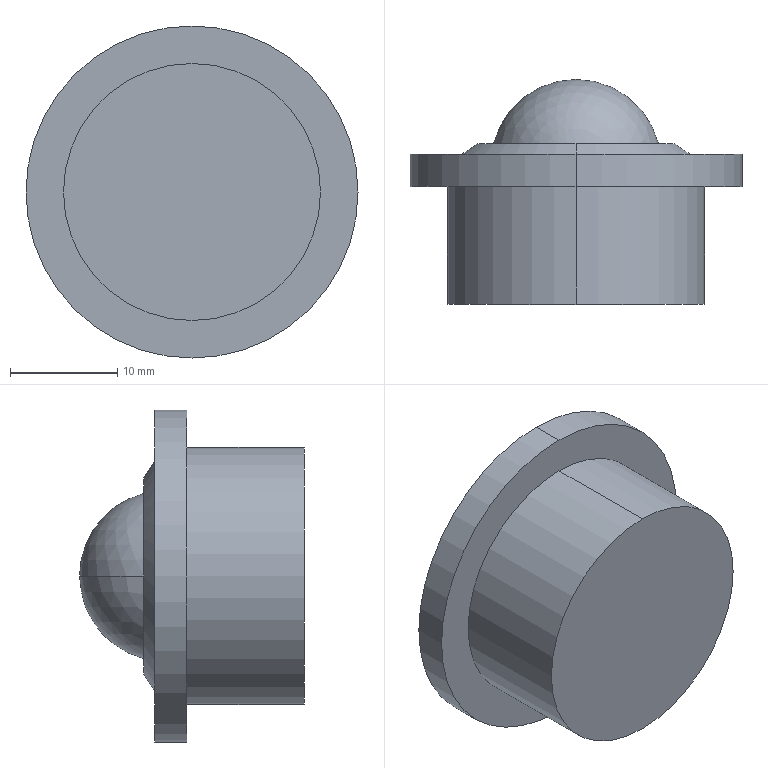Part | STEP file | Universal ball bearing H21xD31xh6-40KG | 1 solid | 12 faces | box 31 x 21 x 31 mm | volume 8224 mm3 | cylinder 4 | plane 4 | cone 2 | sphere 2 | commonest cylinder face diameters 24 x2 31 x2
STEP:
#1=CARTESIAN_POINT('',(0.,0.,0.));
#2=DIRECTION('',(0.,0.,1.));
#3=DIRECTION('',(1.,0.,0.));
#4=AXIS2_PLACEMENT_3D('',#1,#2,#3);
#5=CARTESIAN_POINT('',(0.,15.,-9.197));
#6=VERTEX_POINT('',#5);
#7=CARTESIAN_POINT('',(0.,15.,9.197));
#8=VERTEX_POINT('',#7);
#9=CARTESIAN_POINT('',(0.,15.,0.));
#10=DIRECTION('',(0.,-1.,0.));
#11=DIRECTION('',(0.,0.,-1.));
#12=AXIS2_PLACEMENT_3D('',#9,#10,#11);
#13=CIRCLE('',#12,9.197);
#14=CARTESIAN_POINT('',(0.,15.,0.));
#15=DIRECTION('',(0.,-1.,0.));
#16=DIRECTION('',(0.,0.,-1.));
#17=AXIS2_PLACEMENT_3D('',#14,#15,#16);
#18=CONICAL_SURFACE('',#17,9.197,0.9828);
#19=CARTESIAN_POINT('',(0.,0.));
#20=DIRECTION('',(1.,0.));
#21=VECTOR('',#20,1.);
#22=LINE('',#19,#21);
#23=(GEOMETRIC_REPRESENTATION_CONTEXT(2)PARAMETRIC_REPRESENTATION_CONTEXT()REPRESENTATION_CONTEXT('',''));
#24=DEFINITIONAL_REPRESENTATION('',(#22),#23);
#25=PCURVE('',#18,#24);
#26=CARTESIAN_POINT('',(0.,15.,0.));
#27=DIRECTION('',(0.,-1.,0.));
#28=DIRECTION('',(0.,0.,-1.));
#29=AXIS2_PLACEMENT_3D('',#26,#27,#28);
#30=PLANE('',#29);
#31=CARTESIAN_POINT('',(0.,0.));
#32=DIRECTION('',(1.,0.));
#33=AXIS2_PLACEMENT_2D('',#31,#32);
#34=CIRCLE('',#33,9.197);
#35=(GEOMETRIC_REPRESENTATION_CONTEXT(2)PARAMETRIC_REPRESENTATION_CONTEXT()REPRESENTATION_CONTEXT('',''));
#36=DEFINITIONAL_REPRESENTATION('',(#34),#35);
#37=PCURVE('',#30,#36);
#38=SURFACE_CURVE('',#13,(#25,#37),.PCURVE_S1.);
#39=EDGE_CURVE('',#6,#8,#38,.T.);
#40=ORIENTED_EDGE('',*,*,#39,.T.);
#41=CARTESIAN_POINT('',(0.,14.,10.697));
#42=VERTEX_POINT('',#41);
#43=CARTESIAN_POINT('',(0.,15.,9.197));
#44=DIRECTION('',(0.,-0.5547,0.8321));
#45=VECTOR('',#44,1.);
#46=LINE('',#43,#45);
#47=CARTESIAN_POINT('',(3.142,0.));
#48=DIRECTION('',(0.,1.));
#49=VECTOR('',#48,1.);
#50=LINE('',#47,#49);
#51=(GEOMETRIC_REPRESENTATION_CONTEXT(2)PARAMETRIC_REPRESENTATION_CONTEXT()REPRESENTATION_CONTEXT('',''));
#52=DEFINITIONAL_REPRESENTATION('',(#50),#51);
#53=PCURVE('',#18,#52);
#54=CARTESIAN_POINT('',(0.,15.,0.));
#55=DIRECTION('',(0.,-1.,0.));
#56=DIRECTION('',(0.,0.,-1.));
#57=AXIS2_PLACEMENT_3D('',#54,#55,#56);
#58=CONICAL_SURFACE('',#57,9.197,0.9828);
#59=CARTESIAN_POINT('',(3.142,0.));
#60=DIRECTION('',(0.,1.));
#61=VECTOR('',#60,1.);
#62=LINE('',#59,#61);
#63=(GEOMETRIC_REPRESENTATION_CONTEXT(2)PARAMETRIC_REPRESENTATION_CONTEXT()REPRESENTATION_CONTEXT('',''));
#64=DEFINITIONAL_REPRESENTATION('',(#62),#63);
#65=PCURVE('',#58,#64);
#66=SURFACE_CURVE('',#46,(#53,#65),.PCURVE_S1.);
#67=EDGE_CURVE('',#8,#42,#66,.T.);
#68=ORIENTED_EDGE('',*,*,#67,.T.);
#69=CARTESIAN_POINT('',(0.,14.,-10.697));
#70=VERTEX_POINT('',#69);
#71=CARTESIAN_POINT('',(0.,14.,0.));
#72=DIRECTION('',(0.,-1.,0.));
#73=DIRECTION('',(0.,0.,-1.));
#74=AXIS2_PLACEMENT_3D('',#71,#72,#73);
#75=CIRCLE('',#74,10.697);
#76=CARTESIAN_POINT('',(0.,1.));
#77=DIRECTION('',(1.,0.));
#78=VECTOR('',#77,1.);
#79=LINE('',#76,#78);
#80=(GEOMETRIC_REPRESENTATION_CONTEXT(2)PARAMETRIC_REPRESENTATION_CONTEXT()REPRESENTATION_CONTEXT('',''));
#81=DEFINITIONAL_REPRESENTATION('',(#79),#80);
#82=PCURVE('',#18,#81);
#83=CARTESIAN_POINT('',(0.,14.,0.));
#84=DIRECTION('',(0.,-1.,0.));
#85=DIRECTION('',(0.,0.,-1.));
#86=AXIS2_PLACEMENT_3D('',#83,#84,#85);
#87=PLANE('',#86);
#88=CARTESIAN_POINT('',(0.,0.));
#89=DIRECTION('',(1.,0.));
#90=AXIS2_PLACEMENT_2D('',#88,#89);
#91=CIRCLE('',#90,10.697);
#92=(GEOMETRIC_REPRESENTATION_CONTEXT(2)PARAMETRIC_REPRESENTATION_CONTEXT()REPRESENTATION_CONTEXT('',''));
#93=DEFINITIONAL_REPRESENTATION('',(#91),#92);
#94=PCURVE('',#87,#93);
#95=SURFACE_CURVE('',#75,(#82,#94),.PCURVE_S1.);
#96=EDGE_CURVE('',#70,#42,#95,.T.);
#97=ORIENTED_EDGE('',*,*,#96,.F.);
#98=CARTESIAN_POINT('',(0.,15.,-9.197));
#99=DIRECTION('',(0.,-0.5547,-0.8321));
#100=VECTOR('',#99,1.);
#101=LINE('',#98,#100);
#102=CARTESIAN_POINT('',(0.,0.));
#103=DIRECTION('',(0.,1.));
#104=VECTOR('',#103,1.);
#105=LINE('',#102,#104);
#106=(GEOMETRIC_REPRESENTATION_CONTEXT(2)PARAMETRIC_REPRESENTATION_CONTEXT()REPRESENTATION_CONTEXT('',''));
#107=DEFINITIONAL_REPRESENTATION('',(#105),#106);
#108=PCURVE('',#18,#107);
#109=CARTESIAN_POINT('',(6.283,0.));
#110=DIRECTION('',(0.,1.));
#111=VECTOR('',#110,1.);
#112=LINE('',#109,#111);
#113=(GEOMETRIC_REPRESENTATION_CONTEXT(2)PARAMETRIC_REPRESENTATION_CONTEXT()REPRESENTATION_CONTEXT('',''));
#114=DEFINITIONAL_REPRESENTATION('',(#112),#113);
#115=PCURVE('',#58,#114);
#116=SURFACE_CURVE('',#101,(#108,#115),.PCURVE_S1.);
#117=EDGE_CURVE('',#6,#70,#116,.T.);
#118=ORIENTED_EDGE('',*,*,#117,.F.);
#119=EDGE_LOOP('',(#40,#68,#97,#118));
#120=FACE_BOUND('',#119,.T.);
#121=ADVANCED_FACE('',(#120),#18,.T.);
#122=CARTESIAN_POINT('',(0.,14.,-15.5));
#123=VERTEX_POINT('',#122);
#124=CARTESIAN_POINT('',(0.,14.,15.5));
#125=VERTEX_POINT('',#124);
#126=CARTESIAN_POINT('',(0.,14.,0.));
#127=DIRECTION('',(0.,-1.,0.));
#128=DIRECTION('',(0.,0.,-1.));
#129=AXIS2_PLACEMENT_3D('',#126,#127,#128);
#130=CIRCLE('',#129,15.5);
#131=CARTESIAN_POINT('',(0.,0.,0.));
#132=DIRECTION('',(0.,-1.,0.));
#133=DIRECTION('',(0.,0.,-1.));
#134=AXIS2_PLACEMENT_3D('',#131,#132,#133);
#135=CYLINDRICAL_SURFACE('',#134,15.5);
#136=CARTESIAN_POINT('',(0.,-14.));
#137=DIRECTION('',(1.,0.));
#138=VECTOR('',#137,1.);
#139=LINE('',#136,#138);
#140=(GEOMETRIC_REPRESENTATION_CONTEXT(2)PARAMETRIC_REPRESENTATION_CONTEXT()REPRESENTATION_CONTEXT('',''));
#141=DEFINITIONAL_REPRESENTATION('',(#139),#140);
#142=PCURVE('',#135,#141);
#143=CARTESIAN_POINT('',(0.,0.));
#144=DIRECTION('',(1.,0.));
#145=AXIS2_PLACEMENT_2D('',#143,#144);
#146=CIRCLE('',#145,15.5);
#147=(GEOMETRIC_REPRESENTATION_CONTEXT(2)PARAMETRIC_REPRESENTATION_CONTEXT()REPRESENTATION_CONTEXT('',''));
#148=DEFINITIONAL_REPRESENTATION('',(#146),#147);
#149=PCURVE('',#87,#148);
#150=SURFACE_CURVE('',#130,(#142,#149),.PCURVE_S1.);
#151=EDGE_CURVE('',#123,#125,#150,.T.);
#152=ORIENTED_EDGE('',*,*,#151,.T.);
#153=CARTESIAN_POINT('',(0.,11.,15.5));
#154=VERTEX_POINT('',#153);
#155=CARTESIAN_POINT('',(0.,0.,15.5));
#156=DIRECTION('',(0.,-1.,0.));
#157=VECTOR('',#156,1.);
#158=LINE('',#155,#157);
#159=CARTESIAN_POINT('',(3.142,0.));
#160=DIRECTION('',(0.,1.));
#161=VECTOR('',#160,1.);
#162=LINE('',#159,#161);
#163=(GEOMETRIC_REPRESENTATION_CONTEXT(2)PARAMETRIC_REPRESENTATION_CONTEXT()REPRESENTATION_CONTEXT('',''));
#164=DEFINITIONAL_REPRESENTATION('',(#162),#163);
#165=PCURVE('',#135,#164);
#166=CARTESIAN_POINT('',(0.,0.,0.));
#167=DIRECTION('',(0.,-1.,0.));
#168=DIRECTION('',(0.,0.,-1.));
#169=AXIS2_PLACEMENT_3D('',#166,#167,#168);
#170=CYLINDRICAL_SURFACE('',#169,15.5);
#171=CARTESIAN_POINT('',(3.142,0.));
#172=DIRECTION('',(0.,1.));
#173=VECTOR('',#172,1.);
#174=LINE('',#171,#173);
#175=(GEOMETRIC_REPRESENTATION_CONTEXT(2)PARAMETRIC_REPRESENTATION_CONTEXT()REPRESENTATION_CONTEXT('',''));
#176=DEFINITIONAL_REPRESENTATION('',(#174),#175);
#177=PCURVE('',#170,#176);
#178=SURFACE_CURVE('',#158,(#165,#177),.PCURVE_S1.);
#179=EDGE_CURVE('',#125,#154,#178,.T.);
#180=ORIENTED_EDGE('',*,*,#179,.T.);
#181=CARTESIAN_POINT('',(0.,11.,-15.5));
#182=VERTEX_POINT('',#181);
#183=CARTESIAN_POINT('',(0.,11.,0.));
#184=DIRECTION('',(0.,-1.,0.));
#185=DIRECTION('',(0.,0.,-1.));
#186=AXIS2_PLACEMENT_3D('',#183,#184,#185);
#187=CIRCLE('',#186,15.5);
#188=CARTESIAN_POINT('',(0.,-11.));
#189=DIRECTION('',(1.,0.));
#190=VECTOR('',#189,1.);
#191=LINE('',#188,#190);
#192=(GEOMETRIC_REPRESENTATION_CONTEXT(2)PARAMETRIC_REPRESENTATION_CONTEXT()REPRESENTATION_CONTEXT('',''));
#193=DEFINITIONAL_REPRESENTATION('',(#191),#192);
#194=PCURVE('',#135,#193);
#195=CARTESIAN_POINT('',(0.,11.,0.));
#196=DIRECTION('',(0.,-1.,0.));
#197=DIRECTION('',(0.,0.,-1.));
#198=AXIS2_PLACEMENT_3D('',#195,#196,#197);
#199=PLANE('',#198);
#200=CARTESIAN_POINT('',(0.,0.));
#201=DIRECTION('',(1.,0.));
#202=AXIS2_PLACEMENT_2D('',#200,#201);
#203=CIRCLE('',#202,15.5);
#204=(GEOMETRIC_REPRESENTATION_CONTEXT(2)PARAMETRIC_REPRESENTATION_CONTEXT()REPRESENTATION_CONTEXT('',''));
#205=DEFINITIONAL_REPRESENTATION('',(#203),#204);
#206=PCURVE('',#199,#205);
#207=SURFACE_CURVE('',#187,(#194,#206),.PCURVE_S1.);
#208=EDGE_CURVE('',#182,#154,#207,.T.);
#209=ORIENTED_EDGE('',*,*,#208,.F.);
#210=CARTESIAN_POINT('',(0.,0.,-15.5));
#211=DIRECTION('',(0.,-1.,0.));
#212=VECTOR('',#211,1.);
#213=LINE('',#210,#212);
#214=CARTESIAN_POINT('',(0.,0.));
#215=DIRECTION('',(0.,1.));
#216=VECTOR('',#215,1.);
#217=LINE('',#214,#216);
#218=(GEOMETRIC_REPRESENTATION_CONTEXT(2)PARAMETRIC_REPRESENTATION_CONTEXT()REPRESENTATION_CONTEXT('',''));
#219=DEFINITIONAL_REPRESENTATION('',(#217),#218);
#220=PCURVE('',#135,#219);
#221=CARTESIAN_POINT('',(6.283,0.));
#222=DIRECTION('',(0.,1.));
#223=VECTOR('',#222,1.);
#224=LINE('',#221,#223);
#225=(GEOMETRIC_REPRESENTATION_CONTEXT(2)PARAMETRIC_REPRESENTATION_CONTEXT()REPRESENTATION_CONTEXT('',''));
#226=DEFINITIONAL_REPRESENTATION('',(#224),#225);
#227=PCURVE('',#170,#226);
#228=SURFACE_CURVE('',#213,(#220,#227),.PCURVE_S1.);
#229=EDGE_CURVE('',#123,#182,#228,.T.);
#230=ORIENTED_EDGE('',*,*,#229,.F.);
#231=EDGE_LOOP('',(#152,#180,#209,#230));
#232=FACE_BOUND('',#231,.T.);
#233=ADVANCED_FACE('',(#232),#135,.T.);
#234=CARTESIAN_POINT('',(0.,11.,-12.));
#235=VERTEX_POINT('',#234);
#236=CARTESIAN_POINT('',(0.,11.,12.));
#237=VERTEX_POINT('',#236);
#238=CARTESIAN_POINT('',(0.,11.,0.));
#239=DIRECTION('',(0.,-1.,0.));
#240=DIRECTION('',(0.,0.,-1.));
#241=AXIS2_PLACEMENT_3D('',#238,#239,#240);
#242=CIRCLE('',#241,12.);
#243=CARTESIAN_POINT('',(0.,0.,0.));
#244=DIRECTION('',(0.,-1.,0.));
#245=DIRECTION('',(0.,0.,-1.));
#246=AXIS2_PLACEMENT_3D('',#243,#244,#245);
#247=CYLINDRICAL_SURFACE('',#246,12.);
#248=CARTESIAN_POINT('',(0.,-11.));
#249=DIRECTION('',(1.,0.));
#250=VECTOR('',#249,1.);
#251=LINE('',#248,#250);
#252=(GEOMETRIC_REPRESENTATION_CONTEXT(2)PARAMETRIC_REPRESENTATION_CONTEXT()REPRESENTATION_CONTEXT('',''));
#253=DEFINITIONAL_REPRESENTATION('',(#251),#252);
#254=PCURVE('',#247,#253);
#255=CARTESIAN_POINT('',(0.,0.));
#256=DIRECTION('',(1.,0.));
#257=AXIS2_PLACEMENT_2D('',#255,#256);
#258=CIRCLE('',#257,12.);
#259=(GEOMETRIC_REPRESENTATION_CONTEXT(2)PARAMETRIC_REPRESENTATION_CONTEXT()REPRESENTATION_CONTEXT('',''));
#260=DEFINITIONAL_REPRESENTATION('',(#258),#259);
#261=PCURVE('',#199,#260);
#262=SURFACE_CURVE('',#242,(#254,#261),.PCURVE_S1.);
#263=EDGE_CURVE('',#235,#237,#262,.T.);
#264=ORIENTED_EDGE('',*,*,#263,.T.);
#265=CARTESIAN_POINT('',(0.,0.,12.));
#266=VERTEX_POINT('',#265);
#267=CARTESIAN_POINT('',(0.,0.,12.));
#268=DIRECTION('',(0.,-1.,0.));
#269=VECTOR('',#268,1.);
#270=LINE('',#267,#269);
#271=CARTESIAN_POINT('',(3.142,0.));
#272=DIRECTION('',(0.,1.));
#273=VECTOR('',#272,1.);
#274=LINE('',#271,#273);
#275=(GEOMETRIC_REPRESENTATION_CONTEXT(2)PARAMETRIC_REPRESENTATION_CONTEXT()REPRESENTATION_CONTEXT('',''));
#276=DEFINITIONAL_REPRESENTATION('',(#274),#275);
#277=PCURVE('',#247,#276);
#278=CARTESIAN_POINT('',(0.,0.,0.));
#279=DIRECTION('',(0.,-1.,0.));
#280=DIRECTION('',(0.,0.,-1.));
#281=AXIS2_PLACEMENT_3D('',#278,#279,#280);
#282=CYLINDRICAL_SURFACE('',#281,12.);
#283=CARTESIAN_POINT('',(3.142,0.));
#284=DIRECTION('',(0.,1.));
#285=VECTOR('',#284,1.);
#286=LINE('',#283,#285);
#287=(GEOMETRIC_REPRESENTATION_CONTEXT(2)PARAMETRIC_REPRESENTATION_CONTEXT()REPRESENTATION_CONTEXT('',''));
#288=DEFINITIONAL_REPRESENTATION('',(#286),#287);
#289=PCURVE('',#282,#288);
#290=SURFACE_CURVE('',#270,(#277,#289),.PCURVE_S1.);
#291=EDGE_CURVE('',#237,#266,#290,.T.);
#292=ORIENTED_EDGE('',*,*,#291,.T.);
#293=CARTESIAN_POINT('',(0.,0.,-12.));
#294=VERTEX_POINT('',#293);
#295=CARTESIAN_POINT('',(0.,0.,0.));
#296=DIRECTION('',(0.,-1.,0.));
#297=DIRECTION('',(0.,0.,-1.));
#298=AXIS2_PLACEMENT_3D('',#295,#296,#297);
#299=CIRCLE('',#298,12.);
#300=CARTESIAN_POINT('',(0.,0.));
#301=DIRECTION('',(1.,0.));
#302=VECTOR('',#301,1.);
#303=LINE('',#300,#302);
#304=(GEOMETRIC_REPRESENTATION_CONTEXT(2)PARAMETRIC_REPRESENTATION_CONTEXT()REPRESENTATION_CONTEXT('',''));
#305=DEFINITIONAL_REPRESENTATION('',(#303),#304);
#306=PCURVE('',#247,#305);
#307=CARTESIAN_POINT('',(0.,0.,0.));
#308=DIRECTION('',(0.,-1.,0.));
#309=DIRECTION('',(0.,0.,-1.));
#310=AXIS2_PLACEMENT_3D('',#307,#308,#309);
#311=PLANE('',#310);
#312=CARTESIAN_POINT('',(0.,0.));
#313=DIRECTION('',(1.,0.));
#314=AXIS2_PLACEMENT_2D('',#312,#313);
#315=CIRCLE('',#314,12.);
#316=(GEOMETRIC_REPRESENTATION_CONTEXT(2)PARAMETRIC_REPRESENTATION_CONTEXT()REPRESENTATION_CONTEXT('',''));
#317=DEFINITIONAL_REPRESENTATION('',(#315),#316);
#318=PCURVE('',#311,#317);
#319=SURFACE_CURVE('',#299,(#306,#318),.PCURVE_S1.);
#320=EDGE_CURVE('',#294,#266,#319,.T.);
#321=ORIENTED_EDGE('',*,*,#320,.F.);
#322=CARTESIAN_POINT('',(0.,0.,-12.));
#323=DIRECTION('',(0.,-1.,0.));
#324=VECTOR('',#323,1.);
#325=LINE('',#322,#324);
#326=CARTESIAN_POINT('',(0.,0.));
#327=DIRECTION('',(0.,1.));
#328=VECTOR('',#327,1.);
#329=LINE('',#326,#328);
#330=(GEOMETRIC_REPRESENTATION_CONTEXT(2)PARAMETRIC_REPRESENTATION_CONTEXT()REPRESENTATION_CONTEXT('',''));
#331=DEFINITIONAL_REPRESENTATION('',(#329),#330);
#332=PCURVE('',#247,#331);
#333=CARTESIAN_POINT('',(6.283,0.));
#334=DIRECTION('',(0.,1.));
#335=VECTOR('',#334,1.);
#336=LINE('',#333,#335);
#337=(GEOMETRIC_REPRESENTATION_CONTEXT(2)PARAMETRIC_REPRESENTATION_CONTEXT()REPRESENTATION_CONTEXT('',''));
#338=DEFINITIONAL_REPRESENTATION('',(#336),#337);
#339=PCURVE('',#282,#338);
#340=SURFACE_CURVE('',#325,(#332,#339),.PCURVE_S1.);
#341=EDGE_CURVE('',#235,#294,#340,.T.);
#342=ORIENTED_EDGE('',*,*,#341,.F.);
#343=EDGE_LOOP('',(#264,#292,#321,#342));
#344=FACE_BOUND('',#343,.T.);
#345=ADVANCED_FACE('',(#344),#247,.T.);
#346=CARTESIAN_POINT('',(0.,21.,0.));
#347=VERTEX_POINT('',#346);
#348=CARTESIAN_POINT('',(7.697,15.,0.));
#349=VERTEX_POINT('',#348);
#350=CARTESIAN_POINT('',(0.,13.062,0.));
#351=DIRECTION('',(0.,0.,-1.));
#352=DIRECTION('',(-1.,0.,0.));
#353=AXIS2_PLACEMENT_3D('',#350,#351,#352);
#354=CIRCLE('',#353,7.938);
#355=CARTESIAN_POINT('',(0.,13.062,0.));
#356=DIRECTION('',(0.,0.,1.));
#357=DIRECTION('',(1.,0.,0.));
#358=AXIS2_PLACEMENT_3D('',#355,#356,#357);
#359=SPHERICAL_SURFACE('',#358,7.938);
#360=CARTESIAN_POINT('',(3.142,0.));
#361=DIRECTION('',(-1.,0.));
#362=VECTOR('',#361,1.);
#363=LINE('',#360,#362);
#364=(GEOMETRIC_REPRESENTATION_CONTEXT(2)PARAMETRIC_REPRESENTATION_CONTEXT()REPRESENTATION_CONTEXT('',''));
#365=DEFINITIONAL_REPRESENTATION('',(#363),#364);
#366=PCURVE('',#359,#365);
#367=CARTESIAN_POINT('',(0.,13.062,0.));
#368=DIRECTION('',(0.,0.,1.));
#369=DIRECTION('',(1.,0.,0.));
#370=AXIS2_PLACEMENT_3D('',#367,#368,#369);
#371=SPHERICAL_SURFACE('',#370,7.938);
#372=CARTESIAN_POINT('',(3.142,0.));
#373=DIRECTION('',(-1.,0.));
#374=VECTOR('',#373,1.);
#375=LINE('',#372,#374);
#376=(GEOMETRIC_REPRESENTATION_CONTEXT(2)PARAMETRIC_REPRESENTATION_CONTEXT()REPRESENTATION_CONTEXT('',''));
#377=DEFINITIONAL_REPRESENTATION('',(#375),#376);
#378=PCURVE('',#371,#377);
#379=SURFACE_CURVE('',#354,(#366,#378),.PCURVE_S1.);
#380=EDGE_CURVE('',#347,#349,#379,.T.);
#381=ORIENTED_EDGE('',*,*,#380,.F.);
#382=CARTESIAN_POINT('',(-7.697,15.,0.));
#383=VERTEX_POINT('',#382);
#384=CARTESIAN_POINT('',(0.,13.062,0.));
#385=DIRECTION('',(0.,0.,1.));
#386=DIRECTION('',(1.,0.,0.));
#387=AXIS2_PLACEMENT_3D('',#384,#385,#386);
#388=CIRCLE('',#387,7.938);
#389=CARTESIAN_POINT('',(0.,0.));
#390=DIRECTION('',(1.,0.));
#391=VECTOR('',#390,1.);
#392=LINE('',#389,#391);
#393=(GEOMETRIC_REPRESENTATION_CONTEXT(2)PARAMETRIC_REPRESENTATION_CONTEXT()REPRESENTATION_CONTEXT('',''));
#394=DEFINITIONAL_REPRESENTATION('',(#392),#393);
#395=PCURVE('',#359,#394);
#396=CARTESIAN_POINT('',(0.,0.));
#397=DIRECTION('',(1.,0.));
#398=VECTOR('',#397,1.);
#399=LINE('',#396,#398);
#400=(GEOMETRIC_REPRESENTATION_CONTEXT(2)PARAMETRIC_REPRESENTATION_CONTEXT()REPRESENTATION_CONTEXT('',''));
#401=DEFINITIONAL_REPRESENTATION('',(#399),#400);
#402=PCURVE('',#371,#401);
#403=SURFACE_CURVE('',#388,(#395,#402),.PCURVE_S1.);
#404=EDGE_CURVE('',#347,#383,#403,.T.);
#405=ORIENTED_EDGE('',*,*,#404,.T.);
#406=CARTESIAN_POINT('',(0.,15.,0.));
#407=DIRECTION('',(0.,-1.,0.));
#408=DIRECTION('',(0.,0.,-1.));
#409=AXIS2_PLACEMENT_3D('',#406,#407,#408);
#410=CIRCLE('',#409,7.697);
#411=CARTESIAN_POINT('',(0.2466,0.));
#412=CARTESIAN_POINT('',(0.2466,0.04616));
#413=CARTESIAN_POINT('',(0.2482,0.1385));
#414=CARTESIAN_POINT('',(0.2556,0.2768));
#415=CARTESIAN_POINT('',(0.2688,0.4147));
#416=CARTESIAN_POINT('',(0.2891,0.552));
#417=CARTESIAN_POINT('',(0.3192,0.6883));
#418=CARTESIAN_POINT('',(0.3633,0.823));
#419=CARTESIAN_POINT('',(0.4295,0.9549));
#420=CARTESIAN_POINT('',(0.5331,1.082));
#421=CARTESIAN_POINT('',(0.7068,1.199));
#422=CARTESIAN_POINT('',(1.015,1.295));
#423=CARTESIAN_POINT('',(1.571,1.339));
#424=CARTESIAN_POINT('',(2.127,1.295));
#425=CARTESIAN_POINT('',(2.435,1.199));
#426=CARTESIAN_POINT('',(2.609,1.082));
#427=CARTESIAN_POINT('',(2.712,0.9549));
#428=CARTESIAN_POINT('',(2.778,0.823));
#429=CARTESIAN_POINT('',(2.822,0.6883));
#430=CARTESIAN_POINT('',(2.852,0.552));
#431=CARTESIAN_POINT('',(2.873,0.4147));
#432=CARTESIAN_POINT('',(2.886,0.2768));
#433=CARTESIAN_POINT('',(2.893,0.1385));
#434=CARTESIAN_POINT('',(2.895,0.04616));
#435=CARTESIAN_POINT('',(2.895,0.));
#436=B_SPLINE_CURVE_WITH_KNOTS('',3,(#411,#412,#413,#414,#415,#416,#417,#418,#419,#420,#421,#422,#423,#424,#425,#426,#427,#428,#429,#430,#431,#432,#433,#434,#435),.UNSPECIFIED.,.F.,.F.,(4,1,1,1,1,1,1,1,1,1,1,1,1,1,1,1,1,1,1,1,1,1,4),(1.571,1.714,1.856,1.999,2.142,2.285,2.428,2.57,2.713,2.856,2.999,3.142,3.284,3.427,3.57,3.713,3.856,3.998,4.141,4.284,4.427,4.57,4.712),.QUASI_UNIFORM_KNOTS.);
#437=(GEOMETRIC_REPRESENTATION_CONTEXT(2)PARAMETRIC_REPRESENTATION_CONTEXT()REPRESENTATION_CONTEXT('',''));
#438=DEFINITIONAL_REPRESENTATION('',(#436),#437);
#439=PCURVE('',#359,#438);
#440=CARTESIAN_POINT('',(0.,0.));
#441=DIRECTION('',(1.,0.));
#442=AXIS2_PLACEMENT_2D('',#440,#441);
#443=CIRCLE('',#442,7.697);
#444=(GEOMETRIC_REPRESENTATION_CONTEXT(2)PARAMETRIC_REPRESENTATION_CONTEXT()REPRESENTATION_CONTEXT('',''));
#445=DEFINITIONAL_REPRESENTATION('',(#443),#444);
#446=PCURVE('',#30,#445);
#447=SURFACE_CURVE('',#410,(#439,#446),.PCURVE_S1.);
#448=EDGE_CURVE('',#349,#383,#447,.T.);
#449=ORIENTED_EDGE('',*,*,#448,.F.);
#450=EDGE_LOOP('',(#381,#405,#449));
#451=FACE_BOUND('',#450,.T.);
#452=ADVANCED_FACE('',(#451),#359,.T.);
#453=ORIENTED_EDGE('',*,*,#39,.F.);
#454=CARTESIAN_POINT('',(0.,15.,0.));
#455=DIRECTION('',(0.,-1.,0.));
#456=DIRECTION('',(0.,0.,-1.));
#457=AXIS2_PLACEMENT_3D('',#454,#455,#456);
#458=CIRCLE('',#457,9.197);
#459=CARTESIAN_POINT('',(0.,0.));
#460=DIRECTION('',(1.,0.));
#461=AXIS2_PLACEMENT_2D('',#459,#460);
#462=CIRCLE('',#461,9.197);
#463=(GEOMETRIC_REPRESENTATION_CONTEXT(2)PARAMETRIC_REPRESENTATION_CONTEXT()REPRESENTATION_CONTEXT('',''));
#464=DEFINITIONAL_REPRESENTATION('',(#462),#463);
#465=PCURVE('',#30,#464);
#466=CARTESIAN_POINT('',(0.,0.));
#467=DIRECTION('',(1.,0.));
#468=VECTOR('',#467,1.);
#469=LINE('',#466,#468);
#470=(GEOMETRIC_REPRESENTATION_CONTEXT(2)PARAMETRIC_REPRESENTATION_CONTEXT()REPRESENTATION_CONTEXT('',''));
#471=DEFINITIONAL_REPRESENTATION('',(#469),#470);
#472=PCURVE('',#58,#471);
#473=SURFACE_CURVE('',#458,(#465,#472),.PCURVE_S1.);
#474=EDGE_CURVE('',#8,#6,#473,.T.);
#475=ORIENTED_EDGE('',*,*,#474,.F.);
#476=EDGE_LOOP('',(#453,#475));
#477=FACE_BOUND('',#476,.T.);
#478=ORIENTED_EDGE('',*,*,#448,.T.);
#479=CARTESIAN_POINT('',(0.,15.,0.));
#480=DIRECTION('',(0.,-1.,0.));
#481=DIRECTION('',(0.,0.,-1.));
#482=AXIS2_PLACEMENT_3D('',#479,#480,#481);
#483=CIRCLE('',#482,7.697);
#484=CARTESIAN_POINT('',(0.,0.));
#485=DIRECTION('',(1.,0.));
#486=AXIS2_PLACEMENT_2D('',#484,#485);
#487=CIRCLE('',#486,7.697);
#488=(GEOMETRIC_REPRESENTATION_CONTEXT(2)PARAMETRIC_REPRESENTATION_CONTEXT()REPRESENTATION_CONTEXT('',''));
#489=DEFINITIONAL_REPRESENTATION('',(#487),#488);
#490=PCURVE('',#30,#489);
#491=CARTESIAN_POINT('',(2.895,0.));
#492=CARTESIAN_POINT('',(2.895,-0.04616));
#493=CARTESIAN_POINT('',(2.893,-0.1385));
#494=CARTESIAN_POINT('',(2.886,-0.2768));
#495=CARTESIAN_POINT('',(2.873,-0.4147));
#496=CARTESIAN_POINT('',(2.852,-0.552));
#497=CARTESIAN_POINT('',(2.822,-0.6883));
#498=CARTESIAN_POINT('',(2.778,-0.823));
#499=CARTESIAN_POINT('',(2.712,-0.9549));
#500=CARTESIAN_POINT('',(2.609,-1.082));
#501=CARTESIAN_POINT('',(2.435,-1.199));
#502=CARTESIAN_POINT('',(2.127,-1.295));
#503=CARTESIAN_POINT('',(1.571,-1.339));
#504=CARTESIAN_POINT('',(1.015,-1.295));
#505=CARTESIAN_POINT('',(0.7068,-1.199));
#506=CARTESIAN_POINT('',(0.5331,-1.082));
#507=CARTESIAN_POINT('',(0.4295,-0.9549));
#508=CARTESIAN_POINT('',(0.3633,-0.823));
#509=CARTESIAN_POINT('',(0.3192,-0.6883));
#510=CARTESIAN_POINT('',(0.2891,-0.552));
#511=CARTESIAN_POINT('',(0.2688,-0.4147));
#512=CARTESIAN_POINT('',(0.2556,-0.2768));
#513=CARTESIAN_POINT('',(0.2482,-0.1385));
#514=CARTESIAN_POINT('',(0.2466,-0.04616));
#515=CARTESIAN_POINT('',(0.2466,0.));
#516=B_SPLINE_CURVE_WITH_KNOTS('',3,(#491,#492,#493,#494,#495,#496,#497,#498,#499,#500,#501,#502,#503,#504,#505,#506,#507,#508,#509,#510,#511,#512,#513,#514,#515),.UNSPECIFIED.,.F.,.F.,(4,1,1,1,1,1,1,1,1,1,1,1,1,1,1,1,1,1,1,1,1,1,4),(4.712,4.855,4.998,5.141,5.284,5.426,5.569,5.712,5.855,5.998,6.14,6.283,6.426,6.569,6.712,6.854,6.997,7.14,7.283,7.426,7.568,7.711,7.854),.QUASI_UNIFORM_KNOTS.);
#517=(GEOMETRIC_REPRESENTATION_CONTEXT(2)PARAMETRIC_REPRESENTATION_CONTEXT()REPRESENTATION_CONTEXT('',''));
#518=DEFINITIONAL_REPRESENTATION('',(#516),#517);
#519=PCURVE('',#371,#518);
#520=SURFACE_CURVE('',#483,(#490,#519),.PCURVE_S1.);
#521=EDGE_CURVE('',#383,#349,#520,.T.);
#522=ORIENTED_EDGE('',*,*,#521,.T.);
#523=EDGE_LOOP('',(#478,#522));
#524=FACE_BOUND('',#523,.T.);
#525=ADVANCED_FACE('',(#477,#524),#30,.F.);
#526=ORIENTED_EDGE('',*,*,#404,.F.);
#527=ORIENTED_EDGE('',*,*,#380,.T.);
#528=ORIENTED_EDGE('',*,*,#521,.F.);
#529=EDGE_LOOP('',(#526,#527,#528));
#530=FACE_BOUND('',#529,.T.);
#531=ADVANCED_FACE('',(#530),#371,.T.);
#532=ORIENTED_EDGE('',*,*,#320,.T.);
#533=CARTESIAN_POINT('',(0.,0.,0.));
#534=DIRECTION('',(0.,-1.,0.));
#535=DIRECTION('',(0.,0.,-1.));
#536=AXIS2_PLACEMENT_3D('',#533,#534,#535);
#537=CIRCLE('',#536,12.);
#538=CARTESIAN_POINT('',(0.,0.));
#539=DIRECTION('',(1.,0.));
#540=AXIS2_PLACEMENT_2D('',#538,#539);
#541=CIRCLE('',#540,12.);
#542=(GEOMETRIC_REPRESENTATION_CONTEXT(2)PARAMETRIC_REPRESENTATION_CONTEXT()REPRESENTATION_CONTEXT('',''));
#543=DEFINITIONAL_REPRESENTATION('',(#541),#542);
#544=PCURVE('',#311,#543);
#545=CARTESIAN_POINT('',(0.,0.));
#546=DIRECTION('',(1.,0.));
#547=VECTOR('',#546,1.);
#548=LINE('',#545,#547);
#549=(GEOMETRIC_REPRESENTATION_CONTEXT(2)PARAMETRIC_REPRESENTATION_CONTEXT()REPRESENTATION_CONTEXT('',''));
#550=DEFINITIONAL_REPRESENTATION('',(#548),#549);
#551=PCURVE('',#282,#550);
#552=SURFACE_CURVE('',#537,(#544,#551),.PCURVE_S1.);
#553=EDGE_CURVE('',#266,#294,#552,.T.);
#554=ORIENTED_EDGE('',*,*,#553,.T.);
#555=EDGE_LOOP('',(#532,#554));
#556=FACE_BOUND('',#555,.T.);
#557=ADVANCED_FACE('',(#556),#311,.T.);
#558=ORIENTED_EDGE('',*,*,#291,.F.);
#559=CARTESIAN_POINT('',(0.,11.,0.));
#560=DIRECTION('',(0.,-1.,0.));
#561=DIRECTION('',(0.,0.,-1.));
#562=AXIS2_PLACEMENT_3D('',#559,#560,#561);
#563=CIRCLE('',#562,12.);
#564=CARTESIAN_POINT('',(0.,-11.));
#565=DIRECTION('',(1.,0.));
#566=VECTOR('',#565,1.);
#567=LINE('',#564,#566);
#568=(GEOMETRIC_REPRESENTATION_CONTEXT(2)PARAMETRIC_REPRESENTATION_CONTEXT()REPRESENTATION_CONTEXT('',''));
#569=DEFINITIONAL_REPRESENTATION('',(#567),#568);
#570=PCURVE('',#282,#569);
#571=CARTESIAN_POINT('',(0.,0.));
#572=DIRECTION('',(1.,0.));
#573=AXIS2_PLACEMENT_2D('',#571,#572);
#574=CIRCLE('',#573,12.);
#575=(GEOMETRIC_REPRESENTATION_CONTEXT(2)PARAMETRIC_REPRESENTATION_CONTEXT()REPRESENTATION_CONTEXT('',''));
#576=DEFINITIONAL_REPRESENTATION('',(#574),#575);
#577=PCURVE('',#199,#576);
#578=SURFACE_CURVE('',#563,(#570,#577),.PCURVE_S1.);
#579=EDGE_CURVE('',#237,#235,#578,.T.);
#580=ORIENTED_EDGE('',*,*,#579,.T.);
#581=ORIENTED_EDGE('',*,*,#341,.T.);
#582=ORIENTED_EDGE('',*,*,#553,.F.);
#583=EDGE_LOOP('',(#558,#580,#581,#582));
#584=FACE_BOUND('',#583,.T.);
#585=ADVANCED_FACE('',(#584),#282,.T.);
#586=ORIENTED_EDGE('',*,*,#208,.T.);
#587=CARTESIAN_POINT('',(0.,11.,0.));
#588=DIRECTION('',(0.,-1.,0.));
#589=DIRECTION('',(0.,0.,-1.));
#590=AXIS2_PLACEMENT_3D('',#587,#588,#589);
#591=CIRCLE('',#590,15.5);
#592=CARTESIAN_POINT('',(0.,0.));
#593=DIRECTION('',(1.,0.));
#594=AXIS2_PLACEMENT_2D('',#592,#593);
#595=CIRCLE('',#594,15.5);
#596=(GEOMETRIC_REPRESENTATION_CONTEXT(2)PARAMETRIC_REPRESENTATION_CONTEXT()REPRESENTATION_CONTEXT('',''));
#597=DEFINITIONAL_REPRESENTATION('',(#595),#596);
#598=PCURVE('',#199,#597);
#599=CARTESIAN_POINT('',(0.,-11.));
#600=DIRECTION('',(1.,0.));
#601=VECTOR('',#600,1.);
#602=LINE('',#599,#601);
#603=(GEOMETRIC_REPRESENTATION_CONTEXT(2)PARAMETRIC_REPRESENTATION_CONTEXT()REPRESENTATION_CONTEXT('',''));
#604=DEFINITIONAL_REPRESENTATION('',(#602),#603);
#605=PCURVE('',#170,#604);
#606=SURFACE_CURVE('',#591,(#598,#605),.PCURVE_S1.);
#607=EDGE_CURVE('',#154,#182,#606,.T.);
#608=ORIENTED_EDGE('',*,*,#607,.T.);
#609=EDGE_LOOP('',(#586,#608));
#610=FACE_BOUND('',#609,.T.);
#611=ORIENTED_EDGE('',*,*,#263,.F.);
#612=ORIENTED_EDGE('',*,*,#579,.F.);
#613=EDGE_LOOP('',(#611,#612));
#614=FACE_BOUND('',#613,.T.);
#615=ADVANCED_FACE('',(#610,#614),#199,.T.);
#616=ORIENTED_EDGE('',*,*,#179,.F.);
#617=CARTESIAN_POINT('',(0.,14.,0.));
#618=DIRECTION('',(0.,-1.,0.));
#619=DIRECTION('',(0.,0.,-1.));
#620=AXIS2_PLACEMENT_3D('',#617,#618,#619);
#621=CIRCLE('',#620,15.5);
#622=CARTESIAN_POINT('',(0.,-14.));
#623=DIRECTION('',(1.,0.));
#624=VECTOR('',#623,1.);
#625=LINE('',#622,#624);
#626=(GEOMETRIC_REPRESENTATION_CONTEXT(2)PARAMETRIC_REPRESENTATION_CONTEXT()REPRESENTATION_CONTEXT('',''));
#627=DEFINITIONAL_REPRESENTATION('',(#625),#626);
#628=PCURVE('',#170,#627);
#629=CARTESIAN_POINT('',(0.,0.));
#630=DIRECTION('',(1.,0.));
#631=AXIS2_PLACEMENT_2D('',#629,#630);
#632=CIRCLE('',#631,15.5);
#633=(GEOMETRIC_REPRESENTATION_CONTEXT(2)PARAMETRIC_REPRESENTATION_CONTEXT()REPRESENTATION_CONTEXT('',''));
#634=DEFINITIONAL_REPRESENTATION('',(#632),#633);
#635=PCURVE('',#87,#634);
#636=SURFACE_CURVE('',#621,(#628,#635),.PCURVE_S1.);
#637=EDGE_CURVE('',#125,#123,#636,.T.);
#638=ORIENTED_EDGE('',*,*,#637,.T.);
#639=ORIENTED_EDGE('',*,*,#229,.T.);
#640=ORIENTED_EDGE('',*,*,#607,.F.);
#641=EDGE_LOOP('',(#616,#638,#639,#640));
#642=FACE_BOUND('',#641,.T.);
#643=ADVANCED_FACE('',(#642),#170,.T.);
#644=ORIENTED_EDGE('',*,*,#151,.F.);
#645=ORIENTED_EDGE('',*,*,#637,.F.);
#646=EDGE_LOOP('',(#644,#645));
#647=FACE_BOUND('',#646,.T.);
#648=ORIENTED_EDGE('',*,*,#96,.T.);
#649=CARTESIAN_POINT('',(0.,14.,0.));
#650=DIRECTION('',(0.,-1.,0.));
#651=DIRECTION('',(0.,0.,-1.));
#652=AXIS2_PLACEMENT_3D('',#649,#650,#651);
#653=CIRCLE('',#652,10.697);
#654=CARTESIAN_POINT('',(0.,0.));
#655=DIRECTION('',(1.,0.));
#656=AXIS2_PLACEMENT_2D('',#654,#655);
#657=CIRCLE('',#656,10.697);
#658=(GEOMETRIC_REPRESENTATION_CONTEXT(2)PARAMETRIC_REPRESENTATION_CONTEXT()REPRESENTATION_CONTEXT('',''));
#659=DEFINITIONAL_REPRESENTATION('',(#657),#658);
#660=PCURVE('',#87,#659);
#661=CARTESIAN_POINT('',(0.,1.));
#662=DIRECTION('',(1.,0.));
#663=VECTOR('',#662,1.);
#664=LINE('',#661,#663);
#665=(GEOMETRIC_REPRESENTATION_CONTEXT(2)PARAMETRIC_REPRESENTATION_CONTEXT()REPRESENTATION_CONTEXT('',''));
#666=DEFINITIONAL_REPRESENTATION('',(#664),#665);
#667=PCURVE('',#58,#666);
#668=SURFACE_CURVE('',#653,(#660,#667),.PCURVE_S1.);
#669=EDGE_CURVE('',#42,#70,#668,.T.);
#670=ORIENTED_EDGE('',*,*,#669,.T.);
#671=EDGE_LOOP('',(#648,#670));
#672=FACE_BOUND('',#671,.T.);
#673=ADVANCED_FACE('',(#647,#672),#87,.F.);
#674=ORIENTED_EDGE('',*,*,#67,.F.);
#675=ORIENTED_EDGE('',*,*,#474,.T.);
#676=ORIENTED_EDGE('',*,*,#117,.T.);
#677=ORIENTED_EDGE('',*,*,#669,.F.);
#678=EDGE_LOOP('',(#674,#675,#676,#677));
#679=FACE_BOUND('',#678,.T.);
#680=ADVANCED_FACE('',(#679),#58,.T.);
#681=CLOSED_SHELL('',(#121,#233,#345,#452,#525,#531,#557,#585,#615,#643,#673,#680));
#682=MANIFOLD_SOLID_BREP('',#681);
#683=(LENGTH_UNIT()NAMED_UNIT(*)SI_UNIT(.MILLI.,.METRE.));
#684=UNCERTAINTY_MEASURE_WITH_UNIT(LENGTH_MEASURE(0.0000001),#683,'','');
#685=(NAMED_UNIT(*)PLANE_ANGLE_UNIT()SI_UNIT($,.RADIAN.));
#686=(NAMED_UNIT(*)SI_UNIT($,.STERADIAN.)SOLID_ANGLE_UNIT());
#687=(GEOMETRIC_REPRESENTATION_CONTEXT(3)GLOBAL_UNCERTAINTY_ASSIGNED_CONTEXT((#684))GLOBAL_UNIT_ASSIGNED_CONTEXT((#683,#685,#686))REPRESENTATION_CONTEXT('',''));
#688=ADVANCED_BREP_SHAPE_REPRESENTATION('',(#4,#682),#687);